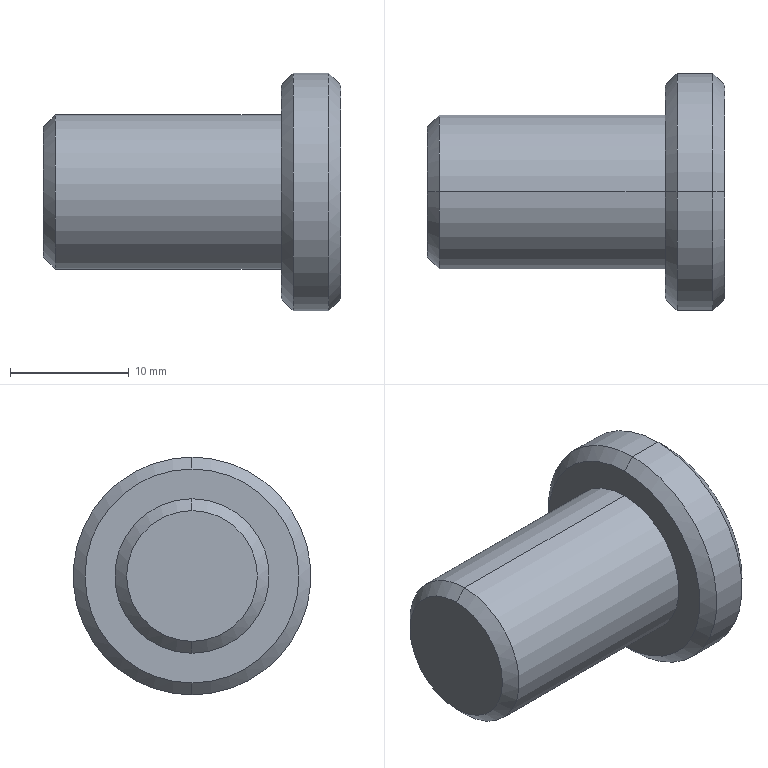Part | SolidWorks | features Chamfer 1, Revolution 1 | 1 solid | 13 faces | box 25 x 20 x 20 mm | volume 4145 mm3 | cone 6 | cylinder 4 | plane 3 | commonest cylinder face diameters 13 x2 20 x2
STEP:
#1=CARTESIAN_POINT('',(236.937,63.731,5.5));
#2=VERTEX_POINT('',#1);
#3=CARTESIAN_POINT('',(236.937,63.731,-5.5));
#4=VERTEX_POINT('',#3);
#5=CARTESIAN_POINT('',(236.937,63.731,0.));
#6=DIRECTION('',(-1.,0.,0.));
#7=DIRECTION('',(0.,0.,-1.));
#8=AXIS2_PLACEMENT_3D('',#5,#6,#7);
#9=CIRCLE('',#8,5.5);
#10=EDGE_CURVE('',#2,#4,#9,.T.);
#11=ORIENTED_EDGE('',*,*,#10,.F.);
#12=CARTESIAN_POINT('',(237.937,63.731,6.5));
#13=VERTEX_POINT('',#12);
#14=CARTESIAN_POINT('',(236.937,63.731,5.5));
#15=DIRECTION('',(0.7071,0.,0.7071));
#16=VECTOR('',#15,1000.);
#17=LINE('',#14,#16);
#18=EDGE_CURVE('',#2,#13,#17,.T.);
#19=ORIENTED_EDGE('',*,*,#18,.T.);
#20=CARTESIAN_POINT('',(237.937,63.731,-6.5));
#21=VERTEX_POINT('',#20);
#22=CARTESIAN_POINT('',(237.937,63.731,0.));
#23=DIRECTION('',(1.,0.,0.));
#24=DIRECTION('',(0.,0.,-1.));
#25=AXIS2_PLACEMENT_3D('',#22,#23,#24);
#26=CIRCLE('',#25,6.5);
#27=EDGE_CURVE('',#21,#13,#26,.T.);
#28=ORIENTED_EDGE('',*,*,#27,.F.);
#29=CARTESIAN_POINT('',(236.937,63.731,-5.5));
#30=DIRECTION('',(0.7071,0.,-0.7071));
#31=VECTOR('',#30,1000.);
#32=LINE('',#29,#31);
#33=EDGE_CURVE('',#4,#21,#32,.T.);
#34=ORIENTED_EDGE('',*,*,#33,.F.);
#35=EDGE_LOOP('',(#11,#19,#28,#34));
#36=FACE_OUTER_BOUND('',#35,.T.);
#37=CARTESIAN_POINT('',(236.937,63.731,0.));
#38=DIRECTION('',(1.,0.,0.));
#39=DIRECTION('',(0.,0.,-1.));
#40=AXIS2_PLACEMENT_3D('',#37,#38,#39);
#41=CONICAL_SURFACE('',#40,5.5,0.7854);
#42=ADVANCED_FACE('',(#36),#41,.T.);
#43=CARTESIAN_POINT('',(256.937,63.731,9.));
#44=VERTEX_POINT('',#43);
#45=CARTESIAN_POINT('',(256.937,63.731,-9.));
#46=VERTEX_POINT('',#45);
#47=CARTESIAN_POINT('',(256.937,63.731,0.));
#48=DIRECTION('',(-1.,0.,0.));
#49=DIRECTION('',(0.,0.,-1.));
#50=AXIS2_PLACEMENT_3D('',#47,#48,#49);
#51=CIRCLE('',#50,9.);
#52=EDGE_CURVE('',#44,#46,#51,.T.);
#53=ORIENTED_EDGE('',*,*,#52,.F.);
#54=CARTESIAN_POINT('',(257.937,63.731,10.));
#55=VERTEX_POINT('',#54);
#56=CARTESIAN_POINT('',(256.937,63.731,9.));
#57=DIRECTION('',(0.7071,0.,0.7071));
#58=VECTOR('',#57,1000.);
#59=LINE('',#56,#58);
#60=EDGE_CURVE('',#44,#55,#59,.T.);
#61=ORIENTED_EDGE('',*,*,#60,.T.);
#62=CARTESIAN_POINT('',(257.937,63.731,-10.));
#63=VERTEX_POINT('',#62);
#64=CARTESIAN_POINT('',(257.937,63.731,0.));
#65=DIRECTION('',(1.,0.,0.));
#66=DIRECTION('',(0.,0.,-1.));
#67=AXIS2_PLACEMENT_3D('',#64,#65,#66);
#68=CIRCLE('',#67,10.);
#69=EDGE_CURVE('',#63,#55,#68,.T.);
#70=ORIENTED_EDGE('',*,*,#69,.F.);
#71=CARTESIAN_POINT('',(256.937,63.731,-9.));
#72=DIRECTION('',(0.7071,0.,-0.7071));
#73=VECTOR('',#72,1000.);
#74=LINE('',#71,#73);
#75=EDGE_CURVE('',#46,#63,#74,.T.);
#76=ORIENTED_EDGE('',*,*,#75,.F.);
#77=EDGE_LOOP('',(#53,#61,#70,#76));
#78=FACE_OUTER_BOUND('',#77,.T.);
#79=CARTESIAN_POINT('',(256.937,63.731,0.));
#80=DIRECTION('',(1.,0.,0.));
#81=DIRECTION('',(0.,0.,-1.));
#82=AXIS2_PLACEMENT_3D('',#79,#80,#81);
#83=CONICAL_SURFACE('',#82,9.,0.7854);
#84=ADVANCED_FACE('',(#78),#83,.T.);
#85=CARTESIAN_POINT('',(261.937,63.731,-9.));
#86=VERTEX_POINT('',#85);
#87=CARTESIAN_POINT('',(261.937,63.731,9.));
#88=VERTEX_POINT('',#87);
#89=CARTESIAN_POINT('',(261.937,63.731,0.));
#90=DIRECTION('',(1.,0.,0.));
#91=DIRECTION('',(0.,0.,1.));
#92=AXIS2_PLACEMENT_3D('',#89,#90,#91);
#93=CIRCLE('',#92,9.);
#94=EDGE_CURVE('',#86,#88,#93,.T.);
#95=ORIENTED_EDGE('',*,*,#94,.F.);
#96=CARTESIAN_POINT('',(260.937,63.731,-10.));
#97=VERTEX_POINT('',#96);
#98=CARTESIAN_POINT('',(260.937,63.731,-10.));
#99=DIRECTION('',(-0.7071,0.,-0.7071));
#100=VECTOR('',#99,1000.);
#101=LINE('',#98,#100);
#102=EDGE_CURVE('',#86,#97,#101,.T.);
#103=ORIENTED_EDGE('',*,*,#102,.T.);
#104=CARTESIAN_POINT('',(260.937,63.731,10.));
#105=VERTEX_POINT('',#104);
#106=CARTESIAN_POINT('',(260.937,63.731,0.));
#107=DIRECTION('',(-1.,0.,0.));
#108=DIRECTION('',(0.,0.,1.));
#109=AXIS2_PLACEMENT_3D('',#106,#107,#108);
#110=CIRCLE('',#109,10.);
#111=EDGE_CURVE('',#105,#97,#110,.T.);
#112=ORIENTED_EDGE('',*,*,#111,.F.);
#113=CARTESIAN_POINT('',(260.937,63.731,10.));
#114=DIRECTION('',(-0.7071,0.,0.7071));
#115=VECTOR('',#114,1000.);
#116=LINE('',#113,#115);
#117=EDGE_CURVE('',#88,#105,#116,.T.);
#118=ORIENTED_EDGE('',*,*,#117,.F.);
#119=EDGE_LOOP('',(#95,#103,#112,#118));
#120=FACE_OUTER_BOUND('',#119,.T.);
#121=CARTESIAN_POINT('',(260.937,63.731,0.));
#122=DIRECTION('',(-1.,0.,0.));
#123=DIRECTION('',(0.,0.,1.));
#124=AXIS2_PLACEMENT_3D('',#121,#122,#123);
#125=CONICAL_SURFACE('',#124,10.,0.7854);
#126=ADVANCED_FACE('',(#120),#125,.T.);
#127=CARTESIAN_POINT('',(256.937,63.731,6.5));
#128=VERTEX_POINT('',#127);
#129=CARTESIAN_POINT('',(256.937,63.731,-6.5));
#130=VERTEX_POINT('',#129);
#131=CARTESIAN_POINT('',(256.937,63.731,0.));
#132=DIRECTION('',(-1.,0.,0.));
#133=DIRECTION('',(0.,0.,1.));
#134=AXIS2_PLACEMENT_3D('',#131,#132,#133);
#135=CIRCLE('',#134,6.5);
#136=EDGE_CURVE('',#128,#130,#135,.T.);
#137=ORIENTED_EDGE('',*,*,#136,.T.);
#138=CARTESIAN_POINT('',(232.937,63.731,-6.5));
#139=DIRECTION('',(-1.,0.,0.));
#140=VECTOR('',#139,1000.);
#141=LINE('',#138,#140);
#142=EDGE_CURVE('',#130,#21,#141,.T.);
#143=ORIENTED_EDGE('',*,*,#142,.T.);
#144=ORIENTED_EDGE('',*,*,#27,.T.);
#145=CARTESIAN_POINT('',(232.937,63.731,6.5));
#146=DIRECTION('',(-1.,0.,0.));
#147=VECTOR('',#146,1000.);
#148=LINE('',#145,#147);
#149=EDGE_CURVE('',#128,#13,#148,.T.);
#150=ORIENTED_EDGE('',*,*,#149,.F.);
#151=EDGE_LOOP('',(#137,#143,#144,#150));
#152=FACE_OUTER_BOUND('',#151,.T.);
#153=CARTESIAN_POINT('',(232.937,63.731,0.));
#154=DIRECTION('',(-1.,0.,0.));
#155=DIRECTION('',(0.,0.,1.));
#156=AXIS2_PLACEMENT_3D('',#153,#154,#155);
#157=CYLINDRICAL_SURFACE('',#156,6.5);
#158=ADVANCED_FACE('',(#152),#157,.T.);
#159=ORIENTED_EDGE('',*,*,#111,.T.);
#160=CARTESIAN_POINT('',(232.937,63.731,-10.));
#161=DIRECTION('',(-1.,0.,0.));
#162=VECTOR('',#161,1000.);
#163=LINE('',#160,#162);
#164=EDGE_CURVE('',#97,#63,#163,.T.);
#165=ORIENTED_EDGE('',*,*,#164,.T.);
#166=ORIENTED_EDGE('',*,*,#69,.T.);
#167=CARTESIAN_POINT('',(232.937,63.731,10.));
#168=DIRECTION('',(-1.,0.,0.));
#169=VECTOR('',#168,1000.);
#170=LINE('',#167,#169);
#171=EDGE_CURVE('',#105,#55,#170,.T.);
#172=ORIENTED_EDGE('',*,*,#171,.F.);
#173=EDGE_LOOP('',(#159,#165,#166,#172));
#174=FACE_OUTER_BOUND('',#173,.T.);
#175=CARTESIAN_POINT('',(232.937,63.731,0.));
#176=DIRECTION('',(-1.,0.,0.));
#177=DIRECTION('',(0.,0.,1.));
#178=AXIS2_PLACEMENT_3D('',#175,#176,#177);
#179=CYLINDRICAL_SURFACE('',#178,10.);
#180=ADVANCED_FACE('',(#174),#179,.T.);
#181=CARTESIAN_POINT('',(236.937,63.731,0.));
#182=DIRECTION('',(-1.,0.,0.));
#183=DIRECTION('',(0.,0.,-1.));
#184=AXIS2_PLACEMENT_3D('',#181,#182,#183);
#185=CIRCLE('',#184,5.5);
#186=EDGE_CURVE('',#4,#2,#185,.T.);
#187=ORIENTED_EDGE('',*,*,#186,.T.);
#188=ORIENTED_EDGE('',*,*,#10,.T.);
#189=EDGE_LOOP('',(#187,#188));
#190=FACE_OUTER_BOUND('',#189,.T.);
#191=CARTESIAN_POINT('',(236.937,70.231,0.));
#192=DIRECTION('',(1.,0.,0.));
#193=DIRECTION('',(0.,0.,-1.));
#194=AXIS2_PLACEMENT_3D('',#191,#192,#193);
#195=PLANE('',#194);
#196=ADVANCED_FACE('',(#190),#195,.F.);
#197=CARTESIAN_POINT('',(261.937,63.731,0.));
#198=DIRECTION('',(1.,0.,0.));
#199=DIRECTION('',(0.,0.,1.));
#200=AXIS2_PLACEMENT_3D('',#197,#198,#199);
#201=CIRCLE('',#200,9.);
#202=EDGE_CURVE('',#88,#86,#201,.T.);
#203=ORIENTED_EDGE('',*,*,#202,.T.);
#204=ORIENTED_EDGE('',*,*,#94,.T.);
#205=EDGE_LOOP('',(#203,#204));
#206=FACE_OUTER_BOUND('',#205,.T.);
#207=CARTESIAN_POINT('',(261.937,73.731,0.));
#208=DIRECTION('',(-1.,0.,0.));
#209=DIRECTION('',(0.,0.,1.));
#210=AXIS2_PLACEMENT_3D('',#207,#208,#209);
#211=PLANE('',#210);
#212=ADVANCED_FACE('',(#206),#211,.F.);
#213=ORIENTED_EDGE('',*,*,#164,.F.);
#214=CARTESIAN_POINT('',(260.937,63.731,0.));
#215=DIRECTION('',(-1.,0.,0.));
#216=DIRECTION('',(0.,0.,1.));
#217=AXIS2_PLACEMENT_3D('',#214,#215,#216);
#218=CIRCLE('',#217,10.);
#219=EDGE_CURVE('',#97,#105,#218,.T.);
#220=ORIENTED_EDGE('',*,*,#219,.T.);
#221=ORIENTED_EDGE('',*,*,#171,.T.);
#222=CARTESIAN_POINT('',(257.937,63.731,0.));
#223=DIRECTION('',(1.,0.,0.));
#224=DIRECTION('',(0.,0.,-1.));
#225=AXIS2_PLACEMENT_3D('',#222,#223,#224);
#226=CIRCLE('',#225,10.);
#227=EDGE_CURVE('',#55,#63,#226,.T.);
#228=ORIENTED_EDGE('',*,*,#227,.T.);
#229=EDGE_LOOP('',(#213,#220,#221,#228));
#230=FACE_OUTER_BOUND('',#229,.T.);
#231=CARTESIAN_POINT('',(232.937,63.731,0.));
#232=DIRECTION('',(-1.,0.,0.));
#233=DIRECTION('',(0.,0.,1.));
#234=AXIS2_PLACEMENT_3D('',#231,#232,#233);
#235=CYLINDRICAL_SURFACE('',#234,10.);
#236=ADVANCED_FACE('',(#230),#235,.T.);
#237=CARTESIAN_POINT('',(256.937,63.731,0.));
#238=DIRECTION('',(-1.,0.,0.));
#239=DIRECTION('',(0.,0.,-1.));
#240=AXIS2_PLACEMENT_3D('',#237,#238,#239);
#241=CIRCLE('',#240,9.);
#242=EDGE_CURVE('',#46,#44,#241,.T.);
#243=ORIENTED_EDGE('',*,*,#242,.T.);
#244=ORIENTED_EDGE('',*,*,#52,.T.);
#245=EDGE_LOOP('',(#243,#244));
#246=FACE_OUTER_BOUND('',#245,.T.);
#247=ORIENTED_EDGE('',*,*,#136,.F.);
#248=CARTESIAN_POINT('',(256.937,63.731,0.));
#249=DIRECTION('',(-1.,0.,0.));
#250=DIRECTION('',(0.,0.,1.));
#251=AXIS2_PLACEMENT_3D('',#248,#249,#250);
#252=CIRCLE('',#251,6.5);
#253=EDGE_CURVE('',#130,#128,#252,.T.);
#254=ORIENTED_EDGE('',*,*,#253,.F.);
#255=EDGE_LOOP('',(#247,#254));
#256=FACE_BOUND('',#255,.T.);
#257=CARTESIAN_POINT('',(256.937,70.231,0.));
#258=DIRECTION('',(1.,0.,0.));
#259=DIRECTION('',(0.,0.,-1.));
#260=AXIS2_PLACEMENT_3D('',#257,#258,#259);
#261=PLANE('',#260);
#262=ADVANCED_FACE('',(#246,#256),#261,.F.);
#263=ORIENTED_EDGE('',*,*,#142,.F.);
#264=ORIENTED_EDGE('',*,*,#253,.T.);
#265=ORIENTED_EDGE('',*,*,#149,.T.);
#266=CARTESIAN_POINT('',(237.937,63.731,0.));
#267=DIRECTION('',(1.,0.,0.));
#268=DIRECTION('',(0.,0.,-1.));
#269=AXIS2_PLACEMENT_3D('',#266,#267,#268);
#270=CIRCLE('',#269,6.5);
#271=EDGE_CURVE('',#13,#21,#270,.T.);
#272=ORIENTED_EDGE('',*,*,#271,.T.);
#273=EDGE_LOOP('',(#263,#264,#265,#272));
#274=FACE_OUTER_BOUND('',#273,.T.);
#275=CARTESIAN_POINT('',(232.937,63.731,0.));
#276=DIRECTION('',(-1.,0.,0.));
#277=DIRECTION('',(0.,0.,1.));
#278=AXIS2_PLACEMENT_3D('',#275,#276,#277);
#279=CYLINDRICAL_SURFACE('',#278,6.5);
#280=ADVANCED_FACE('',(#274),#279,.T.);
#281=ORIENTED_EDGE('',*,*,#102,.F.);
#282=ORIENTED_EDGE('',*,*,#202,.F.);
#283=ORIENTED_EDGE('',*,*,#117,.T.);
#284=ORIENTED_EDGE('',*,*,#219,.F.);
#285=EDGE_LOOP('',(#281,#282,#283,#284));
#286=FACE_OUTER_BOUND('',#285,.T.);
#287=CARTESIAN_POINT('',(260.937,63.731,0.));
#288=DIRECTION('',(-1.,0.,0.));
#289=DIRECTION('',(0.,0.,1.));
#290=AXIS2_PLACEMENT_3D('',#287,#288,#289);
#291=CONICAL_SURFACE('',#290,10.,0.7854);
#292=ADVANCED_FACE('',(#286),#291,.T.);
#293=ORIENTED_EDGE('',*,*,#60,.F.);
#294=ORIENTED_EDGE('',*,*,#242,.F.);
#295=ORIENTED_EDGE('',*,*,#75,.T.);
#296=ORIENTED_EDGE('',*,*,#227,.F.);
#297=EDGE_LOOP('',(#293,#294,#295,#296));
#298=FACE_OUTER_BOUND('',#297,.T.);
#299=CARTESIAN_POINT('',(256.937,63.731,0.));
#300=DIRECTION('',(1.,0.,0.));
#301=DIRECTION('',(0.,0.,-1.));
#302=AXIS2_PLACEMENT_3D('',#299,#300,#301);
#303=CONICAL_SURFACE('',#302,9.,0.7854);
#304=ADVANCED_FACE('',(#298),#303,.T.);
#305=ORIENTED_EDGE('',*,*,#18,.F.);
#306=ORIENTED_EDGE('',*,*,#186,.F.);
#307=ORIENTED_EDGE('',*,*,#33,.T.);
#308=ORIENTED_EDGE('',*,*,#271,.F.);
#309=EDGE_LOOP('',(#305,#306,#307,#308));
#310=FACE_OUTER_BOUND('',#309,.T.);
#311=CARTESIAN_POINT('',(236.937,63.731,0.));
#312=DIRECTION('',(1.,0.,0.));
#313=DIRECTION('',(0.,0.,-1.));
#314=AXIS2_PLACEMENT_3D('',#311,#312,#313);
#315=CONICAL_SURFACE('',#314,5.5,0.7854);
#316=ADVANCED_FACE('',(#310),#315,.T.);
#317=CLOSED_SHELL('',(#42,#84,#126,#158,#180,#196,#212,#236,#262,#280,#292,#304,#316));
#318=MANIFOLD_SOLID_BREP('',#317);
#319=CARTESIAN_POINT('',(0.,0.,0.));
#320=DIRECTION('',(0.,0.,1.));
#321=DIRECTION('',(1.,0.,0.));
#322=AXIS2_PLACEMENT_3D('',#319,#320,#321);
#323=(LENGTH_UNIT()NAMED_UNIT(*)SI_UNIT(.MILLI.,.METRE.));
#324=UNCERTAINTY_MEASURE_WITH_UNIT(LENGTH_MEASURE(0.00001),#323,'','');
#325=(NAMED_UNIT(*)PLANE_ANGLE_UNIT()SI_UNIT($,.RADIAN.));
#326=(NAMED_UNIT(*)SI_UNIT($,.STERADIAN.)SOLID_ANGLE_UNIT());
#327=(GEOMETRIC_REPRESENTATION_CONTEXT(3)GLOBAL_UNCERTAINTY_ASSIGNED_CONTEXT((#324))GLOBAL_UNIT_ASSIGNED_CONTEXT((#323,#325,#326))REPRESENTATION_CONTEXT('',''));
#328=ADVANCED_BREP_SHAPE_REPRESENTATION('',(#318,#322),#327);